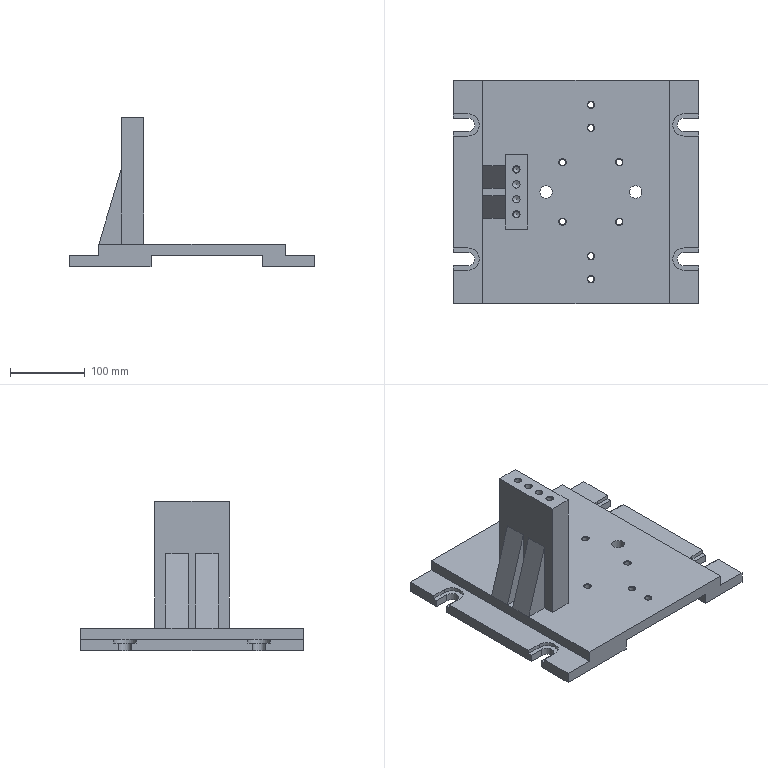Part | NX | features DATUM_CSYS 30, SKETCH 29, EXTRACT_FACE 26, EXTRUDE 15, HOLE PACKAGE 12, SIMPLE HOLE 12, SYMBOLIC_THREAD 10, Instance Feature 9, Mirror Feature 5, Pattern Feature 4, EXTRACT_DATUM_PLANE 2, RIB 2, DATUM_PLANE 1 | 1 solid | 94 faces | box 330 x 300 x 200 mm | volume 2472892 mm3 | plane 50 | cone 22 | cylinder 22 | commonest cylinder face diameters 8.5 x10 18 x4 30 x4 10 x2 17 x2